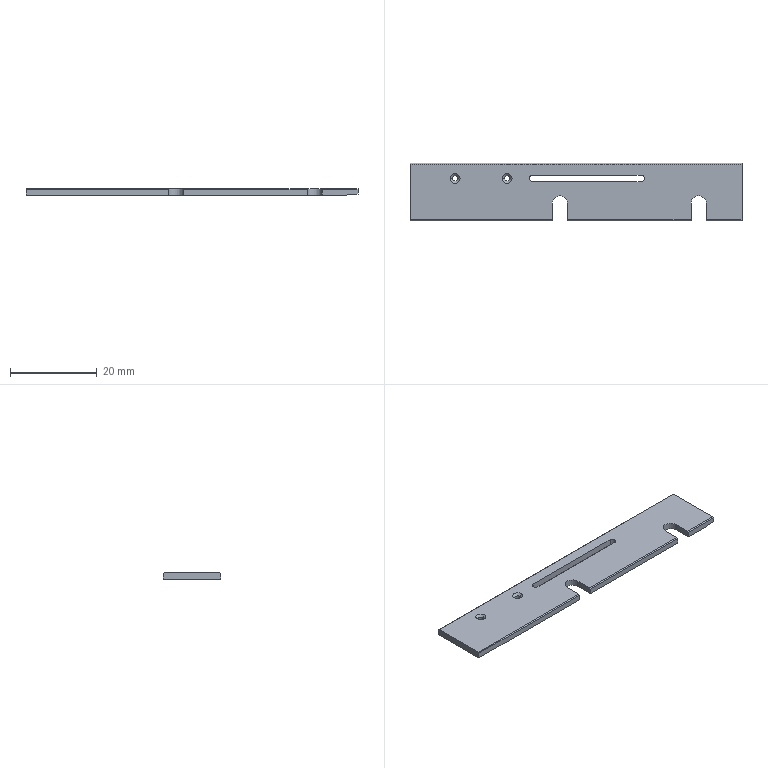Part | NX | 1 solid | 32 faces | box 76.6 x 13.2 x 1.5 mm | volume 1388 mm3 | plane 19 | cylinder 9 | cone 4 | commonest cylinder face diameters 1.3 x4 1.5 x3 3.5 x2
STEP:
#1=CARTESIAN_POINT('',(30.05,-3.5,0.75));
#2=VERTEX_POINT('',#1);
#3=CARTESIAN_POINT('',(30.05,-7.3,0.75));
#4=VERTEX_POINT('',#3);
#5=CARTESIAN_POINT('',(30.05,0.,0.75));
#6=DIRECTION('',(0.,-1.,0.));
#7=VECTOR('',#6,1000.);
#8=LINE('',#5,#7);
#9=EDGE_CURVE('',#2,#4,#8,.T.);
#10=ORIENTED_EDGE('',*,*,#9,.T.);
#11=CARTESIAN_POINT('',(38.3,-7.3,0.75));
#12=VERTEX_POINT('',#11);
#13=CARTESIAN_POINT('',(0.,-7.3,0.75));
#14=DIRECTION('',(-1.,0.,0.));
#15=VECTOR('',#14,1000.);
#16=LINE('',#13,#15);
#17=EDGE_CURVE('',#12,#4,#16,.T.);
#18=ORIENTED_EDGE('',*,*,#17,.F.);
#19=CARTESIAN_POINT('',(38.3,5.5,0.75));
#20=VERTEX_POINT('',#19);
#21=CARTESIAN_POINT('',(38.3,0.,0.75));
#22=DIRECTION('',(0.,-1.,0.));
#23=VECTOR('',#22,1000.);
#24=LINE('',#21,#23);
#25=EDGE_CURVE('',#20,#12,#24,.T.);
#26=ORIENTED_EDGE('',*,*,#25,.F.);
#27=CARTESIAN_POINT('',(-38.3,5.5,0.75));
#28=VERTEX_POINT('',#27);
#29=CARTESIAN_POINT('',(0.,5.5,0.75));
#30=DIRECTION('',(1.,0.,0.));
#31=VECTOR('',#30,1000.);
#32=LINE('',#29,#31);
#33=EDGE_CURVE('',#28,#20,#32,.T.);
#34=ORIENTED_EDGE('',*,*,#33,.F.);
#35=CARTESIAN_POINT('',(-38.3,-7.3,0.75));
#36=VERTEX_POINT('',#35);
#37=CARTESIAN_POINT('',(-38.3,0.,0.75));
#38=DIRECTION('',(0.,1.,0.));
#39=VECTOR('',#38,1000.);
#40=LINE('',#37,#39);
#41=EDGE_CURVE('',#36,#28,#40,.T.);
#42=ORIENTED_EDGE('',*,*,#41,.F.);
#43=CARTESIAN_POINT('',(-5.45,-7.3,0.75));
#44=VERTEX_POINT('',#43);
#45=CARTESIAN_POINT('',(0.,-7.3,0.75));
#46=DIRECTION('',(-1.,0.,0.));
#47=VECTOR('',#46,1000.);
#48=LINE('',#45,#47);
#49=EDGE_CURVE('',#44,#36,#48,.T.);
#50=ORIENTED_EDGE('',*,*,#49,.F.);
#51=CARTESIAN_POINT('',(-5.45,-3.5,0.75));
#52=VERTEX_POINT('',#51);
#53=CARTESIAN_POINT('',(-5.45,0.,0.75));
#54=DIRECTION('',(0.,1.,0.));
#55=VECTOR('',#54,1000.);
#56=LINE('',#53,#55);
#57=EDGE_CURVE('',#44,#52,#56,.T.);
#58=ORIENTED_EDGE('',*,*,#57,.T.);
#59=CARTESIAN_POINT('',(-1.95,-3.5,0.75));
#60=VERTEX_POINT('',#59);
#61=CARTESIAN_POINT('',(-3.7,-3.5,0.75));
#62=DIRECTION('',(0.,0.,-1.));
#63=DIRECTION('',(-1.,0.,0.));
#64=AXIS2_PLACEMENT_3D('',#61,#62,#63);
#65=CIRCLE('',#64,1.75);
#66=EDGE_CURVE('',#52,#60,#65,.T.);
#67=ORIENTED_EDGE('',*,*,#66,.T.);
#68=CARTESIAN_POINT('',(-1.95,-7.3,0.75));
#69=VERTEX_POINT('',#68);
#70=CARTESIAN_POINT('',(-1.95,0.,0.75));
#71=DIRECTION('',(0.,-1.,0.));
#72=VECTOR('',#71,1000.);
#73=LINE('',#70,#72);
#74=EDGE_CURVE('',#60,#69,#73,.T.);
#75=ORIENTED_EDGE('',*,*,#74,.T.);
#76=CARTESIAN_POINT('',(26.55,-7.3,0.75));
#77=VERTEX_POINT('',#76);
#78=CARTESIAN_POINT('',(0.,-7.3,0.75));
#79=DIRECTION('',(-1.,0.,0.));
#80=VECTOR('',#79,1000.);
#81=LINE('',#78,#80);
#82=EDGE_CURVE('',#77,#69,#81,.T.);
#83=ORIENTED_EDGE('',*,*,#82,.F.);
#84=CARTESIAN_POINT('',(26.55,-3.5,0.75));
#85=VERTEX_POINT('',#84);
#86=CARTESIAN_POINT('',(26.55,0.,0.75));
#87=DIRECTION('',(0.,1.,0.));
#88=VECTOR('',#87,1000.);
#89=LINE('',#86,#88);
#90=EDGE_CURVE('',#77,#85,#89,.T.);
#91=ORIENTED_EDGE('',*,*,#90,.T.);
#92=CARTESIAN_POINT('',(28.3,-3.5,0.75));
#93=DIRECTION('',(0.,0.,-1.));
#94=DIRECTION('',(-1.,0.,0.));
#95=AXIS2_PLACEMENT_3D('',#92,#93,#94);
#96=CIRCLE('',#95,1.75);
#97=EDGE_CURVE('',#85,#2,#96,.T.);
#98=ORIENTED_EDGE('',*,*,#97,.T.);
#99=EDGE_LOOP('',(#10,#18,#26,#34,#42,#50,#58,#67,#75,#83,#91,#98));
#100=FACE_BOUND('',#99,.T.);
#101=CARTESIAN_POINT('',(-14.75,2.25,0.75));
#102=VERTEX_POINT('',#101);
#103=CARTESIAN_POINT('',(-17.05,2.25,0.75));
#104=VERTEX_POINT('',#103);
#105=CARTESIAN_POINT('',(-15.9,2.25,0.75));
#106=DIRECTION('',(0.,0.,1.));
#107=DIRECTION('',(1.,0.,0.));
#108=AXIS2_PLACEMENT_3D('',#105,#106,#107);
#109=CIRCLE('',#108,1.15);
#110=EDGE_CURVE('',#102,#104,#109,.T.);
#111=ORIENTED_EDGE('',*,*,#110,.F.);
#112=CARTESIAN_POINT('',(-15.9,2.25,0.75));
#113=DIRECTION('',(0.,0.,1.));
#114=DIRECTION('',(1.,0.,0.));
#115=AXIS2_PLACEMENT_3D('',#112,#113,#114);
#116=CIRCLE('',#115,1.15);
#117=EDGE_CURVE('',#104,#102,#116,.T.);
#118=ORIENTED_EDGE('',*,*,#117,.F.);
#119=EDGE_LOOP('',(#111,#118));
#120=FACE_BOUND('',#119,.T.);
#121=CARTESIAN_POINT('',(15.,1.5,0.75));
#122=VERTEX_POINT('',#121);
#123=CARTESIAN_POINT('',(15.,3.,0.75));
#124=VERTEX_POINT('',#123);
#125=CARTESIAN_POINT('',(15.,2.25,0.75));
#126=DIRECTION('',(0.,0.,1.));
#127=DIRECTION('',(-1.,0.,0.));
#128=AXIS2_PLACEMENT_3D('',#125,#126,#127);
#129=CIRCLE('',#128,0.75);
#130=EDGE_CURVE('',#122,#124,#129,.T.);
#131=ORIENTED_EDGE('',*,*,#130,.F.);
#132=CARTESIAN_POINT('',(-10.,1.5,0.75));
#133=VERTEX_POINT('',#132);
#134=CARTESIAN_POINT('',(0.,1.5,0.75));
#135=DIRECTION('',(1.,0.,0.));
#136=VECTOR('',#135,1000.);
#137=LINE('',#134,#136);
#138=EDGE_CURVE('',#133,#122,#137,.T.);
#139=ORIENTED_EDGE('',*,*,#138,.F.);
#140=CARTESIAN_POINT('',(-10.75,2.25,0.75));
#141=VERTEX_POINT('',#140);
#142=CARTESIAN_POINT('',(-10.,2.25,0.75));
#143=DIRECTION('',(0.,0.,1.));
#144=DIRECTION('',(-1.,0.,0.));
#145=AXIS2_PLACEMENT_3D('',#142,#143,#144);
#146=CIRCLE('',#145,0.75);
#147=EDGE_CURVE('',#141,#133,#146,.T.);
#148=ORIENTED_EDGE('',*,*,#147,.F.);
#149=CARTESIAN_POINT('',(-10.,3.,0.75));
#150=VERTEX_POINT('',#149);
#151=CARTESIAN_POINT('',(-10.,2.25,0.75));
#152=DIRECTION('',(0.,0.,1.));
#153=DIRECTION('',(-1.,0.,0.));
#154=AXIS2_PLACEMENT_3D('',#151,#152,#153);
#155=CIRCLE('',#154,0.75);
#156=EDGE_CURVE('',#150,#141,#155,.T.);
#157=ORIENTED_EDGE('',*,*,#156,.F.);
#158=CARTESIAN_POINT('',(0.,3.,0.75));
#159=DIRECTION('',(-1.,0.,0.));
#160=VECTOR('',#159,1000.);
#161=LINE('',#158,#160);
#162=EDGE_CURVE('',#124,#150,#161,.T.);
#163=ORIENTED_EDGE('',*,*,#162,.F.);
#164=EDGE_LOOP('',(#131,#139,#148,#157,#163));
#165=FACE_BOUND('',#164,.T.);
#166=CARTESIAN_POINT('',(-26.75,2.25,0.75));
#167=VERTEX_POINT('',#166);
#168=CARTESIAN_POINT('',(-29.05,2.25,0.75));
#169=VERTEX_POINT('',#168);
#170=CARTESIAN_POINT('',(-27.9,2.25,0.75));
#171=DIRECTION('',(0.,0.,1.));
#172=DIRECTION('',(1.,0.,0.));
#173=AXIS2_PLACEMENT_3D('',#170,#171,#172);
#174=CIRCLE('',#173,1.15);
#175=EDGE_CURVE('',#167,#169,#174,.T.);
#176=ORIENTED_EDGE('',*,*,#175,.F.);
#177=CARTESIAN_POINT('',(-27.9,2.25,0.75));
#178=DIRECTION('',(0.,0.,1.));
#179=DIRECTION('',(1.,0.,0.));
#180=AXIS2_PLACEMENT_3D('',#177,#178,#179);
#181=CIRCLE('',#180,1.15);
#182=EDGE_CURVE('',#169,#167,#181,.T.);
#183=ORIENTED_EDGE('',*,*,#182,.F.);
#184=EDGE_LOOP('',(#176,#183));
#185=FACE_BOUND('',#184,.T.);
#186=CARTESIAN_POINT('',(0.,0.,0.75));
#187=DIRECTION('',(0.,0.,1.));
#188=DIRECTION('',(1.,0.,0.));
#189=AXIS2_PLACEMENT_3D('',#186,#187,#188);
#190=PLANE('',#189);
#191=ADVANCED_FACE('',(#100,#120,#165,#185),#190,.T.);
#192=CARTESIAN_POINT('',(30.05,-3.5,-0.75));
#193=VERTEX_POINT('',#192);
#194=CARTESIAN_POINT('',(30.05,-7.5,-0.75));
#195=VERTEX_POINT('',#194);
#196=CARTESIAN_POINT('',(30.05,0.,-0.75));
#197=DIRECTION('',(0.,-1.,0.));
#198=VECTOR('',#197,1000.);
#199=LINE('',#196,#198);
#200=EDGE_CURVE('',#193,#195,#199,.T.);
#201=ORIENTED_EDGE('',*,*,#200,.T.);
#202=CARTESIAN_POINT('',(30.05,-7.5,0.55));
#203=VERTEX_POINT('',#202);
#204=CARTESIAN_POINT('',(30.05,-7.5,0.75));
#205=DIRECTION('',(0.,0.,-1.));
#206=VECTOR('',#205,1000.);
#207=LINE('',#204,#206);
#208=EDGE_CURVE('',#203,#195,#207,.T.);
#209=ORIENTED_EDGE('',*,*,#208,.F.);
#210=CARTESIAN_POINT('',(30.05,0.,8.05));
#211=DIRECTION('',(0.,0.7071,0.7071));
#212=VECTOR('',#211,1000.);
#213=LINE('',#210,#212);
#214=EDGE_CURVE('',#203,#4,#213,.T.);
#215=ORIENTED_EDGE('',*,*,#214,.T.);
#216=ORIENTED_EDGE('',*,*,#9,.F.);
#217=CARTESIAN_POINT('',(30.05,-3.5,0.75));
#218=DIRECTION('',(0.,0.,-1.));
#219=VECTOR('',#218,1000.);
#220=LINE('',#217,#219);
#221=EDGE_CURVE('',#2,#193,#220,.T.);
#222=ORIENTED_EDGE('',*,*,#221,.T.);
#223=EDGE_LOOP('',(#201,#209,#215,#216,#222));
#224=FACE_BOUND('',#223,.T.);
#225=CARTESIAN_POINT('',(30.05,-7.5,0.75));
#226=DIRECTION('',(1.,0.,0.));
#227=DIRECTION('',(0.,1.,0.));
#228=AXIS2_PLACEMENT_3D('',#225,#226,#227);
#229=PLANE('',#228);
#230=ADVANCED_FACE('',(#224),#229,.F.);
#231=ORIENTED_EDGE('',*,*,#221,.F.);
#232=ORIENTED_EDGE('',*,*,#97,.F.);
#233=CARTESIAN_POINT('',(26.55,-3.5,-0.75));
#234=VERTEX_POINT('',#233);
#235=CARTESIAN_POINT('',(26.55,-3.5,0.75));
#236=DIRECTION('',(0.,0.,-1.));
#237=VECTOR('',#236,1000.);
#238=LINE('',#235,#237);
#239=EDGE_CURVE('',#85,#234,#238,.T.);
#240=ORIENTED_EDGE('',*,*,#239,.T.);
#241=CARTESIAN_POINT('',(28.3,-3.5,-0.75));
#242=DIRECTION('',(0.,0.,-1.));
#243=DIRECTION('',(-1.,0.,0.));
#244=AXIS2_PLACEMENT_3D('',#241,#242,#243);
#245=CIRCLE('',#244,1.75);
#246=EDGE_CURVE('',#234,#193,#245,.T.);
#247=ORIENTED_EDGE('',*,*,#246,.T.);
#248=EDGE_LOOP('',(#231,#232,#240,#247));
#249=FACE_BOUND('',#248,.T.);
#250=CARTESIAN_POINT('',(28.3,-3.5,0.75));
#251=DIRECTION('',(0.,0.,-1.));
#252=DIRECTION('',(-1.,0.,0.));
#253=AXIS2_PLACEMENT_3D('',#250,#251,#252);
#254=CYLINDRICAL_SURFACE('',#253,1.75);
#255=ADVANCED_FACE('',(#249),#254,.F.);
#256=CARTESIAN_POINT('',(26.55,-7.5,-0.75));
#257=VERTEX_POINT('',#256);
#258=CARTESIAN_POINT('',(26.55,0.,-0.75));
#259=DIRECTION('',(0.,1.,0.));
#260=VECTOR('',#259,1000.);
#261=LINE('',#258,#260);
#262=EDGE_CURVE('',#257,#234,#261,.T.);
#263=ORIENTED_EDGE('',*,*,#262,.T.);
#264=ORIENTED_EDGE('',*,*,#239,.F.);
#265=ORIENTED_EDGE('',*,*,#90,.F.);
#266=CARTESIAN_POINT('',(26.55,-7.5,0.55));
#267=VERTEX_POINT('',#266);
#268=CARTESIAN_POINT('',(26.55,0.,8.05));
#269=DIRECTION('',(0.,-0.7071,-0.7071));
#270=VECTOR('',#269,1000.);
#271=LINE('',#268,#270);
#272=EDGE_CURVE('',#77,#267,#271,.T.);
#273=ORIENTED_EDGE('',*,*,#272,.T.);
#274=CARTESIAN_POINT('',(26.55,-7.5,0.75));
#275=DIRECTION('',(0.,0.,-1.));
#276=VECTOR('',#275,1000.);
#277=LINE('',#274,#276);
#278=EDGE_CURVE('',#267,#257,#277,.T.);
#279=ORIENTED_EDGE('',*,*,#278,.T.);
#280=EDGE_LOOP('',(#263,#264,#265,#273,#279));
#281=FACE_BOUND('',#280,.T.);
#282=CARTESIAN_POINT('',(26.55,-3.5,0.75));
#283=DIRECTION('',(-1.,0.,0.));
#284=DIRECTION('',(0.,0.,1.));
#285=AXIS2_PLACEMENT_3D('',#282,#283,#284);
#286=PLANE('',#285);
#287=ADVANCED_FACE('',(#281),#286,.F.);
#288=CARTESIAN_POINT('',(-1.95,-7.5,0.55));
#289=VERTEX_POINT('',#288);
#290=CARTESIAN_POINT('',(0.,-7.5,0.55));
#291=DIRECTION('',(1.,0.,0.));
#292=VECTOR('',#291,1000.);
#293=LINE('',#290,#292);
#294=EDGE_CURVE('',#289,#267,#293,.T.);
#295=ORIENTED_EDGE('',*,*,#294,.F.);
#296=CARTESIAN_POINT('',(-1.95,-7.5,-0.75));
#297=VERTEX_POINT('',#296);
#298=CARTESIAN_POINT('',(-1.95,-7.5,0.75));
#299=DIRECTION('',(0.,0.,-1.));
#300=VECTOR('',#299,1000.);
#301=LINE('',#298,#300);
#302=EDGE_CURVE('',#289,#297,#301,.T.);
#303=ORIENTED_EDGE('',*,*,#302,.T.);
#304=CARTESIAN_POINT('',(0.,-7.5,-0.75));
#305=DIRECTION('',(-1.,0.,0.));
#306=VECTOR('',#305,1000.);
#307=LINE('',#304,#306);
#308=EDGE_CURVE('',#257,#297,#307,.T.);
#309=ORIENTED_EDGE('',*,*,#308,.F.);
#310=ORIENTED_EDGE('',*,*,#278,.F.);
#311=EDGE_LOOP('',(#295,#303,#309,#310));
#312=FACE_BOUND('',#311,.T.);
#313=CARTESIAN_POINT('',(-38.3,-7.5,-0.75));
#314=DIRECTION('',(0.,-1.,0.));
#315=DIRECTION('',(0.,0.,-1.));
#316=AXIS2_PLACEMENT_3D('',#313,#314,#315);
#317=PLANE('',#316);
#318=ADVANCED_FACE('',(#312),#317,.T.);
#319=CARTESIAN_POINT('',(-1.95,-3.5,-0.75));
#320=VERTEX_POINT('',#319);
#321=CARTESIAN_POINT('',(-1.95,0.,-0.75));
#322=DIRECTION('',(0.,-1.,0.));
#323=VECTOR('',#322,1000.);
#324=LINE('',#321,#323);
#325=EDGE_CURVE('',#320,#297,#324,.T.);
#326=ORIENTED_EDGE('',*,*,#325,.T.);
#327=ORIENTED_EDGE('',*,*,#302,.F.);
#328=CARTESIAN_POINT('',(-1.95,0.,8.05));
#329=DIRECTION('',(0.,0.7071,0.7071));
#330=VECTOR('',#329,1000.);
#331=LINE('',#328,#330);
#332=EDGE_CURVE('',#289,#69,#331,.T.);
#333=ORIENTED_EDGE('',*,*,#332,.T.);
#334=ORIENTED_EDGE('',*,*,#74,.F.);
#335=CARTESIAN_POINT('',(-1.95,-3.5,0.75));
#336=DIRECTION('',(0.,0.,-1.));
#337=VECTOR('',#336,1000.);
#338=LINE('',#335,#337);
#339=EDGE_CURVE('',#60,#320,#338,.T.);
#340=ORIENTED_EDGE('',*,*,#339,.T.);
#341=EDGE_LOOP('',(#326,#327,#333,#334,#340));
#342=FACE_BOUND('',#341,.T.);
#343=CARTESIAN_POINT('',(-1.95,-7.5,0.75));
#344=DIRECTION('',(1.,0.,0.));
#345=DIRECTION('',(0.,1.,0.));
#346=AXIS2_PLACEMENT_3D('',#343,#344,#345);
#347=PLANE('',#346);
#348=ADVANCED_FACE('',(#342),#347,.F.);
#349=ORIENTED_EDGE('',*,*,#339,.F.);
#350=ORIENTED_EDGE('',*,*,#66,.F.);
#351=CARTESIAN_POINT('',(-5.45,-3.5,-0.75));
#352=VERTEX_POINT('',#351);
#353=CARTESIAN_POINT('',(-5.45,-3.5,0.75));
#354=DIRECTION('',(0.,0.,-1.));
#355=VECTOR('',#354,1000.);
#356=LINE('',#353,#355);
#357=EDGE_CURVE('',#52,#352,#356,.T.);
#358=ORIENTED_EDGE('',*,*,#357,.T.);
#359=CARTESIAN_POINT('',(-3.7,-3.5,-0.75));
#360=DIRECTION('',(0.,0.,-1.));
#361=DIRECTION('',(-1.,0.,0.));
#362=AXIS2_PLACEMENT_3D('',#359,#360,#361);
#363=CIRCLE('',#362,1.75);
#364=EDGE_CURVE('',#352,#320,#363,.T.);
#365=ORIENTED_EDGE('',*,*,#364,.T.);
#366=EDGE_LOOP('',(#349,#350,#358,#365));
#367=FACE_BOUND('',#366,.T.);
#368=CARTESIAN_POINT('',(-3.7,-3.5,0.75));
#369=DIRECTION('',(0.,0.,-1.));
#370=DIRECTION('',(-1.,0.,0.));
#371=AXIS2_PLACEMENT_3D('',#368,#369,#370);
#372=CYLINDRICAL_SURFACE('',#371,1.75);
#373=ADVANCED_FACE('',(#367),#372,.F.);
#374=CARTESIAN_POINT('',(-5.45,-7.5,-0.75));
#375=VERTEX_POINT('',#374);
#376=CARTESIAN_POINT('',(-5.45,0.,-0.75));
#377=DIRECTION('',(0.,1.,0.));
#378=VECTOR('',#377,1000.);
#379=LINE('',#376,#378);
#380=EDGE_CURVE('',#375,#352,#379,.T.);
#381=ORIENTED_EDGE('',*,*,#380,.T.);
#382=ORIENTED_EDGE('',*,*,#357,.F.);
#383=ORIENTED_EDGE('',*,*,#57,.F.);
#384=CARTESIAN_POINT('',(-5.45,-7.5,0.55));
#385=VERTEX_POINT('',#384);
#386=CARTESIAN_POINT('',(-5.45,0.,8.05));
#387=DIRECTION('',(0.,-0.7071,-0.7071));
#388=VECTOR('',#387,1000.);
#389=LINE('',#386,#388);
#390=EDGE_CURVE('',#44,#385,#389,.T.);
#391=ORIENTED_EDGE('',*,*,#390,.T.);
#392=CARTESIAN_POINT('',(-5.45,-7.5,0.75));
#393=DIRECTION('',(0.,0.,-1.));
#394=VECTOR('',#393,1000.);
#395=LINE('',#392,#394);
#396=EDGE_CURVE('',#385,#375,#395,.T.);
#397=ORIENTED_EDGE('',*,*,#396,.T.);
#398=EDGE_LOOP('',(#381,#382,#383,#391,#397));
#399=FACE_BOUND('',#398,.T.);
#400=CARTESIAN_POINT('',(-5.45,-3.5,0.75));
#401=DIRECTION('',(-1.,0.,0.));
#402=DIRECTION('',(0.,0.,1.));
#403=AXIS2_PLACEMENT_3D('',#400,#401,#402);
#404=PLANE('',#403);
#405=ADVANCED_FACE('',(#399),#404,.F.);
#406=CARTESIAN_POINT('',(-38.3,-7.5,0.55));
#407=VERTEX_POINT('',#406);
#408=CARTESIAN_POINT('',(0.,-7.5,0.55));
#409=DIRECTION('',(1.,0.,0.));
#410=VECTOR('',#409,1000.);
#411=LINE('',#408,#410);
#412=EDGE_CURVE('',#407,#385,#411,.T.);
#413=ORIENTED_EDGE('',*,*,#412,.F.);
#414=CARTESIAN_POINT('',(-38.3,-7.5,-0.75));
#415=VERTEX_POINT('',#414);
#416=CARTESIAN_POINT('',(-38.3,-7.5,0.));
#417=DIRECTION('',(0.,0.,-1.));
#418=VECTOR('',#417,1000.);
#419=LINE('',#416,#418);
#420=EDGE_CURVE('',#407,#415,#419,.T.);
#421=ORIENTED_EDGE('',*,*,#420,.T.);
#422=CARTESIAN_POINT('',(0.,-7.5,-0.75));
#423=DIRECTION('',(-1.,0.,0.));
#424=VECTOR('',#423,1000.);
#425=LINE('',#422,#424);
#426=EDGE_CURVE('',#375,#415,#425,.T.);
#427=ORIENTED_EDGE('',*,*,#426,.F.);
#428=ORIENTED_EDGE('',*,*,#396,.F.);
#429=EDGE_LOOP('',(#413,#421,#427,#428));
#430=FACE_BOUND('',#429,.T.);
#431=CARTESIAN_POINT('',(-38.3,-7.5,-0.75));
#432=DIRECTION('',(0.,-1.,0.));
#433=DIRECTION('',(0.,0.,-1.));
#434=AXIS2_PLACEMENT_3D('',#431,#432,#433);
#435=PLANE('',#434);
#436=ADVANCED_FACE('',(#430),#435,.T.);
#437=CARTESIAN_POINT('',(-38.3,5.7,-0.75));
#438=VERTEX_POINT('',#437);
#439=CARTESIAN_POINT('',(-38.3,0.,-0.75));
#440=DIRECTION('',(0.,1.,0.));
#441=VECTOR('',#440,1000.);
#442=LINE('',#439,#441);
#443=EDGE_CURVE('',#415,#438,#442,.T.);
#444=ORIENTED_EDGE('',*,*,#443,.F.);
#445=ORIENTED_EDGE('',*,*,#420,.F.);
#446=CARTESIAN_POINT('',(-38.3,0.,8.05));
#447=DIRECTION('',(0.,-0.7071,-0.7071));
#448=VECTOR('',#447,1000.);
#449=LINE('',#446,#448);
#450=EDGE_CURVE('',#36,#407,#449,.T.);
#451=ORIENTED_EDGE('',*,*,#450,.F.);
#452=ORIENTED_EDGE('',*,*,#41,.T.);
#453=CARTESIAN_POINT('',(-38.3,5.7,0.55));
#454=VERTEX_POINT('',#453);
#455=CARTESIAN_POINT('',(-38.3,0.,6.25));
#456=DIRECTION('',(0.,-0.7071,0.7071));
#457=VECTOR('',#456,1000.);
#458=LINE('',#455,#457);
#459=EDGE_CURVE('',#454,#28,#458,.T.);
#460=ORIENTED_EDGE('',*,*,#459,.F.);
#461=CARTESIAN_POINT('',(-38.3,5.7,0.));
#462=DIRECTION('',(0.,0.,-1.));
#463=VECTOR('',#462,1000.);
#464=LINE('',#461,#463);
#465=EDGE_CURVE('',#454,#438,#464,.T.);
#466=ORIENTED_EDGE('',*,*,#465,.T.);
#467=EDGE_LOOP('',(#444,#445,#451,#452,#460,#466));
#468=FACE_BOUND('',#467,.T.);
#469=CARTESIAN_POINT('',(-38.3,7.5,-0.75));
#470=DIRECTION('',(-1.,0.,0.));
#471=DIRECTION('',(0.,0.,1.));
#472=AXIS2_PLACEMENT_3D('',#469,#470,#471);
#473=PLANE('',#472);
#474=ADVANCED_FACE('',(#468),#473,.T.);
#475=CARTESIAN_POINT('',(38.3,5.7,0.55));
#476=VERTEX_POINT('',#475);
#477=CARTESIAN_POINT('',(0.,5.7,0.55));
#478=DIRECTION('',(-1.,0.,0.));
#479=VECTOR('',#478,1000.);
#480=LINE('',#477,#479);
#481=EDGE_CURVE('',#476,#454,#480,.T.);
#482=ORIENTED_EDGE('',*,*,#481,.F.);
#483=CARTESIAN_POINT('',(38.3,5.7,-0.4875));
#484=VERTEX_POINT('',#483);
#485=CARTESIAN_POINT('',(38.3,5.7,0.));
#486=DIRECTION('',(0.,0.,1.));
#487=VECTOR('',#486,1000.);
#488=LINE('',#485,#487);
#489=EDGE_CURVE('',#484,#476,#488,.T.);
#490=ORIENTED_EDGE('',*,*,#489,.F.);
#491=CARTESIAN_POINT('',(35.3,5.7,-0.75));
#492=VERTEX_POINT('',#491);
#493=CARTESIAN_POINT('',(0.,5.7,-3.838));
#494=DIRECTION('',(0.9962,0.,0.08716));
#495=VECTOR('',#494,1000.);
#496=LINE('',#493,#495);
#497=EDGE_CURVE('',#492,#484,#496,.T.);
#498=ORIENTED_EDGE('',*,*,#497,.F.);
#499=CARTESIAN_POINT('',(0.,5.7,-0.75));
#500=DIRECTION('',(1.,0.,0.));
#501=VECTOR('',#500,1000.);
#502=LINE('',#499,#501);
#503=EDGE_CURVE('',#438,#492,#502,.T.);
#504=ORIENTED_EDGE('',*,*,#503,.F.);
#505=ORIENTED_EDGE('',*,*,#465,.F.);
#506=EDGE_LOOP('',(#482,#490,#498,#504,#505));
#507=FACE_BOUND('',#506,.T.);
#508=CARTESIAN_POINT('',(38.3,5.7,-0.75));
#509=DIRECTION('',(0.,1.,0.));
#510=DIRECTION('',(1.,0.,0.));
#511=AXIS2_PLACEMENT_3D('',#508,#509,#510);
#512=PLANE('',#511);
#513=ADVANCED_FACE('',(#507),#512,.T.);
#514=CARTESIAN_POINT('',(35.3,-7.5,-0.75));
#515=VERTEX_POINT('',#514);
#516=CARTESIAN_POINT('',(35.3,0.,-0.75));
#517=DIRECTION('',(0.,-1.,0.));
#518=VECTOR('',#517,1000.);
#519=LINE('',#516,#518);
#520=EDGE_CURVE('',#492,#515,#519,.T.);
#521=ORIENTED_EDGE('',*,*,#520,.F.);
#522=ORIENTED_EDGE('',*,*,#497,.T.);
#523=CARTESIAN_POINT('',(38.3,-7.5,-0.4875));
#524=VERTEX_POINT('',#523);
#525=CARTESIAN_POINT('',(38.3,0.,-0.4875));
#526=DIRECTION('',(0.,-1.,0.));
#527=VECTOR('',#526,1000.);
#528=LINE('',#525,#527);
#529=EDGE_CURVE('',#484,#524,#528,.T.);
#530=ORIENTED_EDGE('',*,*,#529,.T.);
#531=CARTESIAN_POINT('',(0.,-7.5,-3.838));
#532=DIRECTION('',(0.9962,0.,0.08716));
#533=VECTOR('',#532,1000.);
#534=LINE('',#531,#533);
#535=EDGE_CURVE('',#515,#524,#534,.T.);
#536=ORIENTED_EDGE('',*,*,#535,.F.);
#537=EDGE_LOOP('',(#521,#522,#530,#536));
#538=FACE_BOUND('',#537,.T.);
#539=CARTESIAN_POINT('',(35.3,-7.5,-0.75));
#540=DIRECTION('',(0.08716,0.,-0.9962));
#541=DIRECTION('',(0.,-1.,0.));
#542=AXIS2_PLACEMENT_3D('',#539,#540,#541);
#543=PLANE('',#542);
#544=ADVANCED_FACE('',(#538),#543,.T.);
#545=CARTESIAN_POINT('',(38.3,-7.5,0.55));
#546=VERTEX_POINT('',#545);
#547=CARTESIAN_POINT('',(0.,-7.5,0.55));
#548=DIRECTION('',(1.,0.,0.));
#549=VECTOR('',#548,1000.);
#550=LINE('',#547,#549);
#551=EDGE_CURVE('',#203,#546,#550,.T.);
#552=ORIENTED_EDGE('',*,*,#551,.F.);
#553=ORIENTED_EDGE('',*,*,#208,.T.);
#554=CARTESIAN_POINT('',(0.,-7.5,-0.75));
#555=DIRECTION('',(-1.,0.,0.));
#556=VECTOR('',#555,1000.);
#557=LINE('',#554,#556);
#558=EDGE_CURVE('',#515,#195,#557,.T.);
#559=ORIENTED_EDGE('',*,*,#558,.F.);
#560=ORIENTED_EDGE('',*,*,#535,.T.);
#561=CARTESIAN_POINT('',(38.3,-7.5,0.));
#562=DIRECTION('',(0.,0.,1.));
#563=VECTOR('',#562,1000.);
#564=LINE('',#561,#563);
#565=EDGE_CURVE('',#524,#546,#564,.T.);
#566=ORIENTED_EDGE('',*,*,#565,.T.);
#567=EDGE_LOOP('',(#552,#553,#559,#560,#566));
#568=FACE_BOUND('',#567,.T.);
#569=CARTESIAN_POINT('',(-38.3,-7.5,-0.75));
#570=DIRECTION('',(0.,-1.,0.));
#571=DIRECTION('',(0.,0.,-1.));
#572=AXIS2_PLACEMENT_3D('',#569,#570,#571);
#573=PLANE('',#572);
#574=ADVANCED_FACE('',(#568),#573,.T.);
#575=ORIENTED_EDGE('',*,*,#200,.F.);
#576=ORIENTED_EDGE('',*,*,#246,.F.);
#577=ORIENTED_EDGE('',*,*,#262,.F.);
#578=ORIENTED_EDGE('',*,*,#308,.T.);
#579=ORIENTED_EDGE('',*,*,#325,.F.);
#580=ORIENTED_EDGE('',*,*,#364,.F.);
#581=ORIENTED_EDGE('',*,*,#380,.F.);
#582=ORIENTED_EDGE('',*,*,#426,.T.);
#583=ORIENTED_EDGE('',*,*,#443,.T.);
#584=ORIENTED_EDGE('',*,*,#503,.T.);
#585=ORIENTED_EDGE('',*,*,#520,.T.);
#586=ORIENTED_EDGE('',*,*,#558,.T.);
#587=EDGE_LOOP('',(#575,#576,#577,#578,#579,#580,#581,#582,#583,#584,#585,#586));
#588=FACE_BOUND('',#587,.T.);
#589=CARTESIAN_POINT('',(-15.25,2.25,-0.75));
#590=VERTEX_POINT('',#589);
#591=CARTESIAN_POINT('',(-16.55,2.25,-0.75));
#592=VERTEX_POINT('',#591);
#593=CARTESIAN_POINT('',(-15.9,2.25,-0.75));
#594=DIRECTION('',(0.,0.,1.));
#595=DIRECTION('',(1.,0.,0.));
#596=AXIS2_PLACEMENT_3D('',#593,#594,#595);
#597=CIRCLE('',#596,0.65);
#598=EDGE_CURVE('',#590,#592,#597,.T.);
#599=ORIENTED_EDGE('',*,*,#598,.T.);
#600=CARTESIAN_POINT('',(-15.9,2.25,-0.75));
#601=DIRECTION('',(0.,0.,1.));
#602=DIRECTION('',(1.,0.,0.));
#603=AXIS2_PLACEMENT_3D('',#600,#601,#602);
#604=CIRCLE('',#603,0.65);
#605=EDGE_CURVE('',#592,#590,#604,.T.);
#606=ORIENTED_EDGE('',*,*,#605,.T.);
#607=EDGE_LOOP('',(#599,#606));
#608=FACE_BOUND('',#607,.T.);
#609=CARTESIAN_POINT('',(-28.55,2.25,-0.75));
#610=VERTEX_POINT('',#609);
#611=CARTESIAN_POINT('',(-27.25,2.25,-0.75));
#612=VERTEX_POINT('',#611);
#613=CARTESIAN_POINT('',(-27.9,2.25,-0.75));
#614=DIRECTION('',(0.,0.,1.));
#615=DIRECTION('',(1.,0.,0.));
#616=AXIS2_PLACEMENT_3D('',#613,#614,#615);
#617=CIRCLE('',#616,0.65);
#618=EDGE_CURVE('',#610,#612,#617,.T.);
#619=ORIENTED_EDGE('',*,*,#618,.T.);
#620=CARTESIAN_POINT('',(-27.9,2.25,-0.75));
#621=DIRECTION('',(0.,0.,1.));
#622=DIRECTION('',(1.,0.,0.));
#623=AXIS2_PLACEMENT_3D('',#620,#621,#622);
#624=CIRCLE('',#623,0.65);
#625=EDGE_CURVE('',#612,#610,#624,.T.);
#626=ORIENTED_EDGE('',*,*,#625,.T.);
#627=EDGE_LOOP('',(#619,#626));
#628=FACE_BOUND('',#627,.T.);
#629=CARTESIAN_POINT('',(15.,1.5,-0.75));
#630=VERTEX_POINT('',#629);
#631=CARTESIAN_POINT('',(15.,3.,-0.75));
#632=VERTEX_POINT('',#631);
#633=CARTESIAN_POINT('',(15.,2.25,-0.75));
#634=DIRECTION('',(0.,0.,1.));
#635=DIRECTION('',(-1.,0.,0.));
#636=AXIS2_PLACEMENT_3D('',#633,#634,#635);
#637=CIRCLE('',#636,0.75);
#638=EDGE_CURVE('',#630,#632,#637,.T.);
#639=ORIENTED_EDGE('',*,*,#638,.T.);
#640=CARTESIAN_POINT('',(-10.,3.,-0.75));
#641=VERTEX_POINT('',#640);
#642=CARTESIAN_POINT('',(0.,3.,-0.75));
#643=DIRECTION('',(1.,0.,0.));
#644=VECTOR('',#643,1000.);
#645=LINE('',#642,#644);
#646=EDGE_CURVE('',#641,#632,#645,.T.);
#647=ORIENTED_EDGE('',*,*,#646,.F.);
#648=CARTESIAN_POINT('',(-10.75,2.25,-0.75));
#649=VERTEX_POINT('',#648);
#650=CARTESIAN_POINT('',(-10.,2.25,-0.75));
#651=DIRECTION('',(0.,0.,1.));
#652=DIRECTION('',(-1.,0.,0.));
#653=AXIS2_PLACEMENT_3D('',#650,#651,#652);
#654=CIRCLE('',#653,0.75);
#655=EDGE_CURVE('',#641,#649,#654,.T.);
#656=ORIENTED_EDGE('',*,*,#655,.T.);
#657=CARTESIAN_POINT('',(-10.,1.5,-0.75));
#658=VERTEX_POINT('',#657);
#659=CARTESIAN_POINT('',(-10.,2.25,-0.75));
#660=DIRECTION('',(0.,0.,1.));
#661=DIRECTION('',(-1.,0.,0.));
#662=AXIS2_PLACEMENT_3D('',#659,#660,#661);
#663=CIRCLE('',#662,0.75);
#664=EDGE_CURVE('',#649,#658,#663,.T.);
#665=ORIENTED_EDGE('',*,*,#664,.T.);
#666=CARTESIAN_POINT('',(0.,1.5,-0.75));
#667=DIRECTION('',(-1.,0.,0.));
#668=VECTOR('',#667,1000.);
#669=LINE('',#666,#668);
#670=EDGE_CURVE('',#630,#658,#669,.T.);
#671=ORIENTED_EDGE('',*,*,#670,.F.);
#672=EDGE_LOOP('',(#639,#647,#656,#665,#671));
#673=FACE_BOUND('',#672,.T.);
#674=CARTESIAN_POINT('',(0.,0.,-0.75));
#675=DIRECTION('',(0.,0.,1.));
#676=DIRECTION('',(1.,0.,0.));
#677=AXIS2_PLACEMENT_3D('',#674,#675,#676);
#678=PLANE('',#677);
#679=ADVANCED_FACE('',(#588,#608,#628,#673),#678,.F.);
#680=ORIENTED_EDGE('',*,*,#529,.F.);
#681=ORIENTED_EDGE('',*,*,#489,.T.);
#682=CARTESIAN_POINT('',(38.3,0.,6.25));
#683=DIRECTION('',(0.,0.7071,-0.7071));
#684=VECTOR('',#683,1000.);
#685=LINE('',#682,#684);
#686=EDGE_CURVE('',#20,#476,#685,.T.);
#687=ORIENTED_EDGE('',*,*,#686,.F.);
#688=ORIENTED_EDGE('',*,*,#25,.T.);
#689=CARTESIAN_POINT('',(38.3,0.,8.05));
#690=DIRECTION('',(0.,0.7071,0.7071));
#691=VECTOR('',#690,1000.);
#692=LINE('',#689,#691);
#693=EDGE_CURVE('',#546,#12,#692,.T.);
#694=ORIENTED_EDGE('',*,*,#693,.F.);
#695=ORIENTED_EDGE('',*,*,#565,.F.);
#696=EDGE_LOOP('',(#680,#681,#687,#688,#694,#695));
#697=FACE_BOUND('',#696,.T.);
#698=CARTESIAN_POINT('',(38.3,-7.5,-0.75));
#699=DIRECTION('',(1.,0.,0.));
#700=DIRECTION('',(0.,1.,0.));
#701=AXIS2_PLACEMENT_3D('',#698,#699,#700);
#702=PLANE('',#701);
#703=ADVANCED_FACE('',(#697),#702,.T.);
#704=CARTESIAN_POINT('',(-16.55,2.25,0.25));
#705=VERTEX_POINT('',#704);
#706=CARTESIAN_POINT('',(-15.25,2.25,0.25));
#707=VERTEX_POINT('',#706);
#708=CARTESIAN_POINT('',(-15.9,2.25,0.25));
#709=DIRECTION('',(0.,0.,1.));
#710=DIRECTION('',(1.,0.,0.));
#711=AXIS2_PLACEMENT_3D('',#708,#709,#710);
#712=CIRCLE('',#711,0.65);
#713=EDGE_CURVE('',#705,#707,#712,.T.);
#714=ORIENTED_EDGE('',*,*,#713,.F.);
#715=CARTESIAN_POINT('',(-16.8,2.25,0.5));
#716=DIRECTION('',(-0.7071,0.,0.7071));
#717=VECTOR('',#716,1000.);
#718=LINE('',#715,#717);
#719=EDGE_CURVE('',#104,#705,#718,.F.);
#720=ORIENTED_EDGE('',*,*,#719,.F.);
#721=ORIENTED_EDGE('',*,*,#117,.T.);
#722=CARTESIAN_POINT('',(-15.,2.25,0.5));
#723=DIRECTION('',(0.7071,0.,0.7071));
#724=VECTOR('',#723,1000.);
#725=LINE('',#722,#724);
#726=EDGE_CURVE('',#102,#707,#725,.F.);
#727=ORIENTED_EDGE('',*,*,#726,.T.);
#728=EDGE_LOOP('',(#714,#720,#721,#727));
#729=FACE_BOUND('',#728,.T.);
#730=CARTESIAN_POINT('',(-15.9,2.25,0.5));
#731=DIRECTION('',(0.,0.,1.));
#732=DIRECTION('',(1.,0.,0.));
#733=AXIS2_PLACEMENT_3D('',#730,#731,#732);
#734=CONICAL_SURFACE('',#733,0.9,0.7854);
#735=ADVANCED_FACE('',(#729),#734,.F.);
#736=CARTESIAN_POINT('',(-10.75,2.25,0.75));
#737=DIRECTION('',(0.,0.,1.));
#738=VECTOR('',#737,1000.);
#739=LINE('',#736,#738);
#740=EDGE_CURVE('',#649,#141,#739,.T.);
#741=ORIENTED_EDGE('',*,*,#740,.F.);
#742=ORIENTED_EDGE('',*,*,#655,.F.);
#743=CARTESIAN_POINT('',(-10.,3.,0.75));
#744=DIRECTION('',(0.,0.,-1.));
#745=VECTOR('',#744,1000.);
#746=LINE('',#743,#745);
#747=EDGE_CURVE('',#150,#641,#746,.T.);
#748=ORIENTED_EDGE('',*,*,#747,.F.);
#749=ORIENTED_EDGE('',*,*,#156,.T.);
#750=EDGE_LOOP('',(#741,#742,#748,#749));
#751=FACE_BOUND('',#750,.T.);
#752=CARTESIAN_POINT('',(-10.,2.25,0.75));
#753=DIRECTION('',(0.,0.,1.));
#754=DIRECTION('',(-1.,0.,0.));
#755=AXIS2_PLACEMENT_3D('',#752,#753,#754);
#756=CYLINDRICAL_SURFACE('',#755,0.75);
#757=ADVANCED_FACE('',(#751),#756,.F.);
#758=ORIENTED_EDGE('',*,*,#713,.T.);
#759=CARTESIAN_POINT('',(-15.25,2.25,-0.75));
#760=DIRECTION('',(0.,0.,1.));
#761=VECTOR('',#760,1000.);
#762=LINE('',#759,#761);
#763=EDGE_CURVE('',#590,#707,#762,.T.);
#764=ORIENTED_EDGE('',*,*,#763,.F.);
#765=ORIENTED_EDGE('',*,*,#605,.F.);
#766=CARTESIAN_POINT('',(-16.55,2.25,-0.75));
#767=DIRECTION('',(0.,0.,1.));
#768=VECTOR('',#767,1000.);
#769=LINE('',#766,#768);
#770=EDGE_CURVE('',#592,#705,#769,.T.);
#771=ORIENTED_EDGE('',*,*,#770,.T.);
#772=EDGE_LOOP('',(#758,#764,#765,#771));
#773=FACE_BOUND('',#772,.T.);
#774=CARTESIAN_POINT('',(-15.9,2.25,-0.75));
#775=DIRECTION('',(0.,0.,1.));
#776=DIRECTION('',(1.,0.,0.));
#777=AXIS2_PLACEMENT_3D('',#774,#775,#776);
#778=CYLINDRICAL_SURFACE('',#777,0.65);
#779=ADVANCED_FACE('',(#773),#778,.F.);
#780=ORIENTED_EDGE('',*,*,#638,.F.);
#781=CARTESIAN_POINT('',(15.,1.5,0.75));
#782=DIRECTION('',(0.,0.,-1.));
#783=VECTOR('',#782,1000.);
#784=LINE('',#781,#783);
#785=EDGE_CURVE('',#122,#630,#784,.T.);
#786=ORIENTED_EDGE('',*,*,#785,.F.);
#787=ORIENTED_EDGE('',*,*,#130,.T.);
#788=CARTESIAN_POINT('',(15.,3.,-0.75));
#789=DIRECTION('',(0.,0.,1.));
#790=VECTOR('',#789,1000.);
#791=LINE('',#788,#790);
#792=EDGE_CURVE('',#632,#124,#791,.T.);
#793=ORIENTED_EDGE('',*,*,#792,.F.);
#794=EDGE_LOOP('',(#780,#786,#787,#793));
#795=FACE_BOUND('',#794,.T.);
#796=CARTESIAN_POINT('',(15.,2.25,0.75));
#797=DIRECTION('',(0.,0.,1.));
#798=DIRECTION('',(-1.,0.,0.));
#799=AXIS2_PLACEMENT_3D('',#796,#797,#798);
#800=CYLINDRICAL_SURFACE('',#799,0.75);
#801=ADVANCED_FACE('',(#795),#800,.F.);
#802=ORIENTED_EDGE('',*,*,#175,.T.);
#803=CARTESIAN_POINT('',(-28.55,2.25,0.25));
#804=VERTEX_POINT('',#803);
#805=CARTESIAN_POINT('',(-28.8,2.25,0.5));
#806=DIRECTION('',(-0.7071,0.,0.7071));
#807=VECTOR('',#806,1000.);
#808=LINE('',#805,#807);
#809=EDGE_CURVE('',#804,#169,#808,.T.);
#810=ORIENTED_EDGE('',*,*,#809,.F.);
#811=CARTESIAN_POINT('',(-27.25,2.25,0.25));
#812=VERTEX_POINT('',#811);
#813=CARTESIAN_POINT('',(-27.9,2.25,0.25));
#814=DIRECTION('',(0.,0.,1.));
#815=DIRECTION('',(1.,0.,0.));
#816=AXIS2_PLACEMENT_3D('',#813,#814,#815);
#817=CIRCLE('',#816,0.65);
#818=EDGE_CURVE('',#812,#804,#817,.T.);
#819=ORIENTED_EDGE('',*,*,#818,.F.);
#820=CARTESIAN_POINT('',(-27.,2.25,0.5));
#821=DIRECTION('',(0.7071,0.,0.7071));
#822=VECTOR('',#821,1000.);
#823=LINE('',#820,#822);
#824=EDGE_CURVE('',#812,#167,#823,.T.);
#825=ORIENTED_EDGE('',*,*,#824,.T.);
#826=EDGE_LOOP('',(#802,#810,#819,#825));
#827=FACE_BOUND('',#826,.T.);
#828=CARTESIAN_POINT('',(-27.9,2.25,0.5));
#829=DIRECTION('',(0.,0.,1.));
#830=DIRECTION('',(1.,0.,0.));
#831=AXIS2_PLACEMENT_3D('',#828,#829,#830);
#832=CONICAL_SURFACE('',#831,0.9,0.7854);
#833=ADVANCED_FACE('',(#827),#832,.F.);
#834=ORIENTED_EDGE('',*,*,#670,.T.);
#835=CARTESIAN_POINT('',(-10.,1.5,-0.75));
#836=DIRECTION('',(0.,0.,1.));
#837=VECTOR('',#836,1000.);
#838=LINE('',#835,#837);
#839=EDGE_CURVE('',#658,#133,#838,.T.);
#840=ORIENTED_EDGE('',*,*,#839,.T.);
#841=ORIENTED_EDGE('',*,*,#138,.T.);
#842=ORIENTED_EDGE('',*,*,#785,.T.);
#843=EDGE_LOOP('',(#834,#840,#841,#842));
#844=FACE_BOUND('',#843,.T.);
#845=CARTESIAN_POINT('',(-8.,1.5,0.75));
#846=DIRECTION('',(0.,-1.,0.));
#847=DIRECTION('',(0.,0.,-1.));
#848=AXIS2_PLACEMENT_3D('',#845,#846,#847);
#849=PLANE('',#848);
#850=ADVANCED_FACE('',(#844),#849,.F.);
#851=ORIENTED_EDGE('',*,*,#618,.F.);
#852=CARTESIAN_POINT('',(-28.55,2.25,-0.75));
#853=DIRECTION('',(0.,0.,1.));
#854=VECTOR('',#853,1000.);
#855=LINE('',#852,#854);
#856=EDGE_CURVE('',#804,#610,#855,.F.);
#857=ORIENTED_EDGE('',*,*,#856,.F.);
#858=CARTESIAN_POINT('',(-27.9,2.25,0.25));
#859=DIRECTION('',(0.,0.,1.));
#860=DIRECTION('',(1.,0.,0.));
#861=AXIS2_PLACEMENT_3D('',#858,#859,#860);
#862=CIRCLE('',#861,0.65);
#863=EDGE_CURVE('',#804,#812,#862,.T.);
#864=ORIENTED_EDGE('',*,*,#863,.T.);
#865=CARTESIAN_POINT('',(-27.25,2.25,-0.75));
#866=DIRECTION('',(0.,0.,1.));
#867=VECTOR('',#866,1000.);
#868=LINE('',#865,#867);
#869=EDGE_CURVE('',#812,#612,#868,.F.);
#870=ORIENTED_EDGE('',*,*,#869,.T.);
#871=EDGE_LOOP('',(#851,#857,#864,#870));
#872=FACE_BOUND('',#871,.T.);
#873=CARTESIAN_POINT('',(-27.9,2.25,-0.75));
#874=DIRECTION('',(0.,0.,1.));
#875=DIRECTION('',(1.,0.,0.));
#876=AXIS2_PLACEMENT_3D('',#873,#874,#875);
#877=CYLINDRICAL_SURFACE('',#876,0.65);
#878=ADVANCED_FACE('',(#872),#877,.F.);
#879=ORIENTED_EDGE('',*,*,#646,.T.);
#880=ORIENTED_EDGE('',*,*,#792,.T.);
#881=ORIENTED_EDGE('',*,*,#162,.T.);
#882=ORIENTED_EDGE('',*,*,#747,.T.);
#883=EDGE_LOOP('',(#879,#880,#881,#882));
#884=FACE_BOUND('',#883,.T.);
#885=CARTESIAN_POINT('',(15.,3.,0.75));
#886=DIRECTION('',(0.,1.,0.));
#887=DIRECTION('',(1.,0.,0.));
#888=AXIS2_PLACEMENT_3D('',#885,#886,#887);
#889=PLANE('',#888);
#890=ADVANCED_FACE('',(#884),#889,.F.);
#891=ORIENTED_EDGE('',*,*,#481,.T.);
#892=ORIENTED_EDGE('',*,*,#459,.T.);
#893=ORIENTED_EDGE('',*,*,#33,.T.);
#894=ORIENTED_EDGE('',*,*,#686,.T.);
#895=EDGE_LOOP('',(#891,#892,#893,#894));
#896=FACE_BOUND('',#895,.T.);
#897=CARTESIAN_POINT('',(0.,5.6,0.65));
#898=DIRECTION('',(0.,0.7071,0.7071));
#899=DIRECTION('',(1.,0.,0.));
#900=AXIS2_PLACEMENT_3D('',#897,#898,#899);
#901=PLANE('',#900);
#902=ADVANCED_FACE('',(#896),#901,.T.);
#903=ORIENTED_EDGE('',*,*,#294,.T.);
#904=ORIENTED_EDGE('',*,*,#272,.F.);
#905=ORIENTED_EDGE('',*,*,#82,.T.);
#906=ORIENTED_EDGE('',*,*,#332,.F.);
#907=EDGE_LOOP('',(#903,#904,#905,#906));
#908=FACE_BOUND('',#907,.T.);
#909=CARTESIAN_POINT('',(12.3,-7.4,0.65));
#910=DIRECTION('',(0.,-0.7071,0.7071));
#911=DIRECTION('',(-1.,0.,0.));
#912=AXIS2_PLACEMENT_3D('',#909,#910,#911);
#913=PLANE('',#912);
#914=ADVANCED_FACE('',(#908),#913,.T.);
#915=ORIENTED_EDGE('',*,*,#551,.T.);
#916=ORIENTED_EDGE('',*,*,#693,.T.);
#917=ORIENTED_EDGE('',*,*,#17,.T.);
#918=ORIENTED_EDGE('',*,*,#214,.F.);
#919=EDGE_LOOP('',(#915,#916,#917,#918));
#920=FACE_BOUND('',#919,.T.);
#921=CARTESIAN_POINT('',(34.175,-7.4,0.65));
#922=DIRECTION('',(0.,-0.7071,0.7071));
#923=DIRECTION('',(-1.,0.,0.));
#924=AXIS2_PLACEMENT_3D('',#921,#922,#923);
#925=PLANE('',#924);
#926=ADVANCED_FACE('',(#920),#925,.T.);
#927=ORIENTED_EDGE('',*,*,#412,.T.);
#928=ORIENTED_EDGE('',*,*,#390,.F.);
#929=ORIENTED_EDGE('',*,*,#49,.T.);
#930=ORIENTED_EDGE('',*,*,#450,.T.);
#931=EDGE_LOOP('',(#927,#928,#929,#930));
#932=FACE_BOUND('',#931,.T.);
#933=CARTESIAN_POINT('',(-21.875,-7.4,0.65));
#934=DIRECTION('',(0.,-0.7071,0.7071));
#935=DIRECTION('',(-1.,0.,0.));
#936=AXIS2_PLACEMENT_3D('',#933,#934,#935);
#937=PLANE('',#936);
#938=ADVANCED_FACE('',(#932),#937,.T.);
#939=ORIENTED_EDGE('',*,*,#818,.T.);
#940=ORIENTED_EDGE('',*,*,#856,.T.);
#941=ORIENTED_EDGE('',*,*,#625,.F.);
#942=ORIENTED_EDGE('',*,*,#869,.F.);
#943=EDGE_LOOP('',(#939,#940,#941,#942));
#944=FACE_BOUND('',#943,.T.);
#945=CARTESIAN_POINT('',(-27.9,2.25,-0.75));
#946=DIRECTION('',(0.,0.,1.));
#947=DIRECTION('',(1.,0.,0.));
#948=AXIS2_PLACEMENT_3D('',#945,#946,#947);
#949=CYLINDRICAL_SURFACE('',#948,0.65);
#950=ADVANCED_FACE('',(#944),#949,.F.);
#951=ORIENTED_EDGE('',*,*,#110,.T.);
#952=ORIENTED_EDGE('',*,*,#719,.T.);
#953=CARTESIAN_POINT('',(-15.9,2.25,0.25));
#954=DIRECTION('',(0.,0.,1.));
#955=DIRECTION('',(1.,0.,0.));
#956=AXIS2_PLACEMENT_3D('',#953,#954,#955);
#957=CIRCLE('',#956,0.65);
#958=EDGE_CURVE('',#707,#705,#957,.T.);
#959=ORIENTED_EDGE('',*,*,#958,.F.);
#960=ORIENTED_EDGE('',*,*,#726,.F.);
#961=EDGE_LOOP('',(#951,#952,#959,#960));
#962=FACE_BOUND('',#961,.T.);
#963=CARTESIAN_POINT('',(-15.9,2.25,0.5));
#964=DIRECTION('',(0.,0.,1.));
#965=DIRECTION('',(1.,0.,0.));
#966=AXIS2_PLACEMENT_3D('',#963,#964,#965);
#967=CONICAL_SURFACE('',#966,0.9,0.7854);
#968=ADVANCED_FACE('',(#962),#967,.F.);
#969=ORIENTED_EDGE('',*,*,#598,.F.);
#970=ORIENTED_EDGE('',*,*,#763,.T.);
#971=ORIENTED_EDGE('',*,*,#958,.T.);
#972=ORIENTED_EDGE('',*,*,#770,.F.);
#973=EDGE_LOOP('',(#969,#970,#971,#972));
#974=FACE_BOUND('',#973,.T.);
#975=CARTESIAN_POINT('',(-15.9,2.25,-0.75));
#976=DIRECTION('',(0.,0.,1.));
#977=DIRECTION('',(1.,0.,0.));
#978=AXIS2_PLACEMENT_3D('',#975,#976,#977);
#979=CYLINDRICAL_SURFACE('',#978,0.65);
#980=ADVANCED_FACE('',(#974),#979,.F.);
#981=ORIENTED_EDGE('',*,*,#824,.F.);
#982=ORIENTED_EDGE('',*,*,#863,.F.);
#983=ORIENTED_EDGE('',*,*,#809,.T.);
#984=ORIENTED_EDGE('',*,*,#182,.T.);
#985=EDGE_LOOP('',(#981,#982,#983,#984));
#986=FACE_BOUND('',#985,.T.);
#987=CARTESIAN_POINT('',(-27.9,2.25,0.5));
#988=DIRECTION('',(0.,0.,1.));
#989=DIRECTION('',(1.,0.,0.));
#990=AXIS2_PLACEMENT_3D('',#987,#988,#989);
#991=CONICAL_SURFACE('',#990,0.9,0.7854);
#992=ADVANCED_FACE('',(#986),#991,.F.);
#993=ORIENTED_EDGE('',*,*,#664,.F.);
#994=ORIENTED_EDGE('',*,*,#740,.T.);
#995=ORIENTED_EDGE('',*,*,#147,.T.);
#996=ORIENTED_EDGE('',*,*,#839,.F.);
#997=EDGE_LOOP('',(#993,#994,#995,#996));
#998=FACE_BOUND('',#997,.T.);
#999=CARTESIAN_POINT('',(-10.,2.25,0.75));
#1000=DIRECTION('',(0.,0.,1.));
#1001=DIRECTION('',(-1.,0.,0.));
#1002=AXIS2_PLACEMENT_3D('',#999,#1000,#1001);
#1003=CYLINDRICAL_SURFACE('',#1002,0.75);
#1004=ADVANCED_FACE('',(#998),#1003,.F.);
#1005=CLOSED_SHELL('',(#191,#230,#255,#287,#318,#348,#373,#405,#436,#474,#513,#544,#574,#679,#703,#735,#757,#779,#801,#833,#850,#878,#890,#902,#914,#926,#938,#950,#968,#980,#992,#1004));
#1006=MANIFOLD_SOLID_BREP('',#1005);
#1007=(LENGTH_UNIT()NAMED_UNIT(*)SI_UNIT(.MILLI.,.METRE.));
#1008=UNCERTAINTY_MEASURE_WITH_UNIT(LENGTH_MEASURE(0.00001),#1007,'','');
#1009=(NAMED_UNIT(*)PLANE_ANGLE_UNIT()SI_UNIT($,.RADIAN.));
#1010=(NAMED_UNIT(*)SI_UNIT($,.STERADIAN.)SOLID_ANGLE_UNIT());
#1011=(GEOMETRIC_REPRESENTATION_CONTEXT(3)GLOBAL_UNCERTAINTY_ASSIGNED_CONTEXT((#1008))GLOBAL_UNIT_ASSIGNED_CONTEXT((#1007,#1009,#1010))REPRESENTATION_CONTEXT('',''));
#1012=ADVANCED_BREP_SHAPE_REPRESENTATION('',(#1006),#1011);